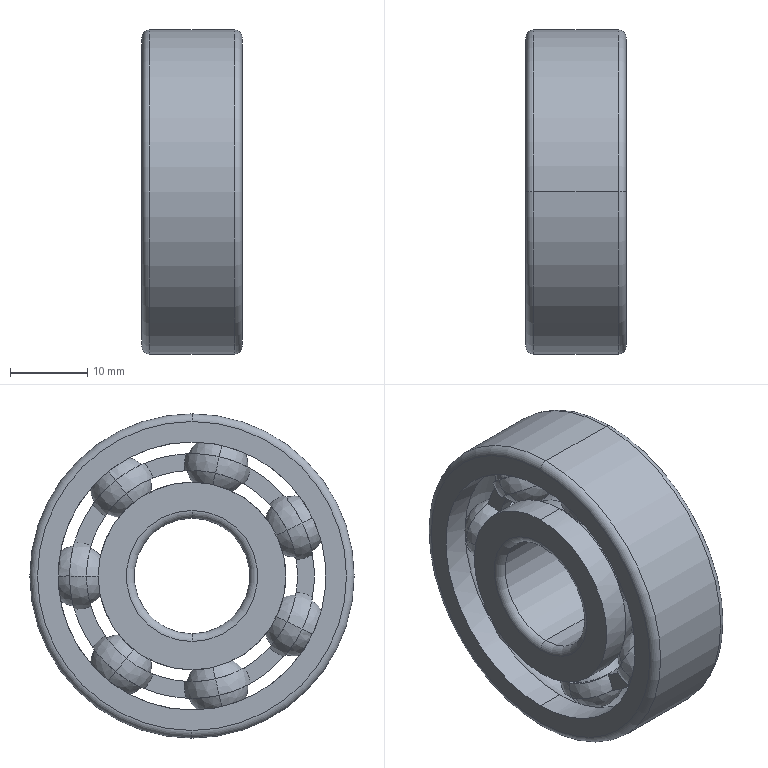Part | STEP file | Bearing 6302 | 1 solid | 122 faces | box 13 x 42 x 42 mm | volume 10445 mm3 | sphere 56 | torus 32 | plane 18 | cylinder 16 | commonest cylinder face diameters 24.3 x4 34.7 x4 15 x2 27.317 x2 31.683 x2 42 x2